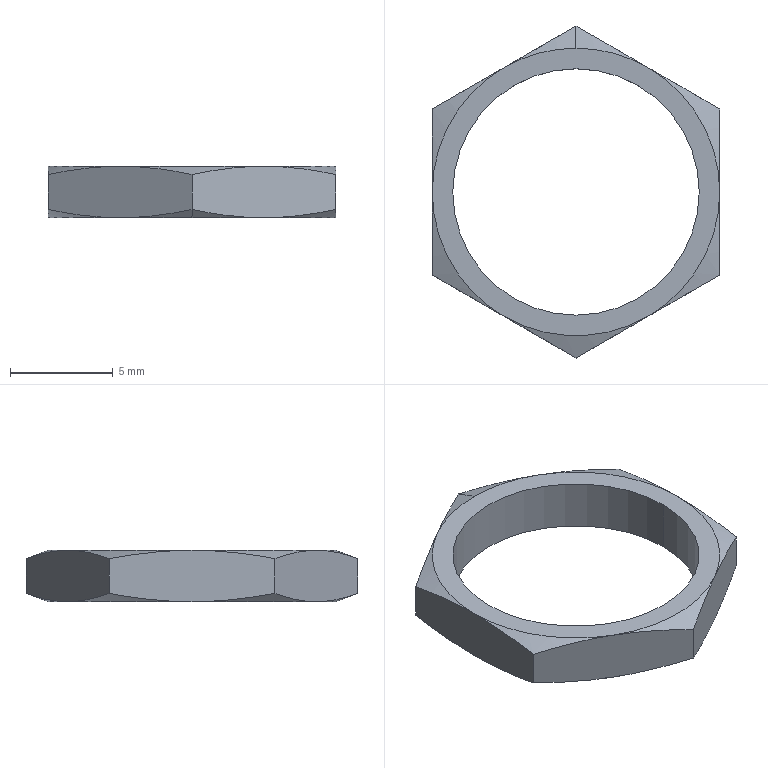Part | SolidWorks | features Extrusion 1, RevCut 1 | 1 solid | 24 faces | box 14 x 16.166 x 2.5 mm | volume 137.79 mm3 | cone 14 | plane 8 | cylinder 2 | commonest cylinder face diameters 12 x2
STEP:
#1=CARTESIAN_POINT('',(-3.5,6.062,2.5));
#2=VERTEX_POINT('',#1);
#3=CARTESIAN_POINT('',(0.,7.,2.5));
#4=VERTEX_POINT('',#3);
#5=CARTESIAN_POINT('',(0.,0.,2.5));
#6=DIRECTION('',(0.,0.,-1.));
#7=DIRECTION('',(0.,1.,0.));
#8=AXIS2_PLACEMENT_3D('',#5,#6,#7);
#9=CIRCLE('',#8,7.);
#10=EDGE_CURVE('',#2,#4,#9,.T.);
#11=ORIENTED_EDGE('',*,*,#10,.T.);
#12=CARTESIAN_POINT('',(0.,8.083,2.1));
#13=VERTEX_POINT('',#12);
#14=CARTESIAN_POINT('',(0.,7.,2.5));
#15=DIRECTION('',(0.,0.9381,-0.3465));
#16=VECTOR('',#15,1000.);
#17=LINE('',#14,#16);
#18=EDGE_CURVE('',#4,#13,#17,.T.);
#19=ORIENTED_EDGE('',*,*,#18,.T.);
#20=CARTESIAN_POINT('',(-3.5,6.062,2.5));
#21=CARTESIAN_POINT('',(-2.917,6.399,2.5));
#22=CARTESIAN_POINT('',(-2.333,6.736,2.463));
#23=CARTESIAN_POINT('',(-1.167,7.409,2.325));
#24=CARTESIAN_POINT('',(-0.5833,7.746,2.224));
#25=CARTESIAN_POINT('',(0.,8.083,2.1));
#26=B_SPLINE_CURVE_WITH_KNOTS('',3,(#20,#21,#22,#23,#24,#25),.UNSPECIFIED.,.F.,.F.,(4,2,4),(0.004042,0.006062,0.008083),.UNSPECIFIED.);
#27=EDGE_CURVE('',#2,#13,#26,.T.);
#28=ORIENTED_EDGE('',*,*,#27,.F.);
#29=EDGE_LOOP('',(#11,#19,#28));
#30=FACE_OUTER_BOUND('',#29,.T.);
#31=CARTESIAN_POINT('',(0.,0.,2.5));
#32=DIRECTION('',(0.,0.,-1.));
#33=DIRECTION('',(0.,1.,0.));
#34=AXIS2_PLACEMENT_3D('',#31,#32,#33);
#35=CONICAL_SURFACE('',#34,7.,1.217);
#36=ADVANCED_FACE('',(#30),#35,.T.);
#37=CARTESIAN_POINT('',(0.,-7.,0.));
#38=VERTEX_POINT('',#37);
#39=CARTESIAN_POINT('',(-3.5,-6.062,0.));
#40=VERTEX_POINT('',#39);
#41=CARTESIAN_POINT('',(0.,0.,0.));
#42=DIRECTION('',(0.,0.,-1.));
#43=DIRECTION('',(0.,1.,0.));
#44=AXIS2_PLACEMENT_3D('',#41,#42,#43);
#45=CIRCLE('',#44,7.);
#46=EDGE_CURVE('',#38,#40,#45,.T.);
#47=ORIENTED_EDGE('',*,*,#46,.F.);
#48=CARTESIAN_POINT('',(0.,-8.083,0.4));
#49=VERTEX_POINT('',#48);
#50=CARTESIAN_POINT('',(0.,-8.083,0.4));
#51=DIRECTION('',(0.,-0.9381,0.3465));
#52=VECTOR('',#51,1000.);
#53=LINE('',#50,#52);
#54=EDGE_CURVE('',#38,#49,#53,.T.);
#55=ORIENTED_EDGE('',*,*,#54,.T.);
#56=CARTESIAN_POINT('',(-3.5,-6.062,0.));
#57=CARTESIAN_POINT('',(-2.917,-6.399,0.));
#58=CARTESIAN_POINT('',(-2.333,-6.736,0.03657));
#59=CARTESIAN_POINT('',(-1.167,-7.409,0.1746));
#60=CARTESIAN_POINT('',(-0.5833,-7.746,0.2756));
#61=CARTESIAN_POINT('',(0.,-8.083,0.4));
#62=B_SPLINE_CURVE_WITH_KNOTS('',3,(#56,#57,#58,#59,#60,#61),.UNSPECIFIED.,.F.,.F.,(4,2,4),(0.004042,0.006062,0.008083),.UNSPECIFIED.);
#63=EDGE_CURVE('',#40,#49,#62,.T.);
#64=ORIENTED_EDGE('',*,*,#63,.F.);
#65=EDGE_LOOP('',(#47,#55,#64));
#66=FACE_OUTER_BOUND('',#65,.T.);
#67=CARTESIAN_POINT('',(0.,0.,0.4));
#68=DIRECTION('',(0.,0.,1.));
#69=DIRECTION('',(0.,-1.,0.));
#70=AXIS2_PLACEMENT_3D('',#67,#68,#69);
#71=CONICAL_SURFACE('',#70,8.083,1.217);
#72=ADVANCED_FACE('',(#66),#71,.T.);
#73=CARTESIAN_POINT('',(-6.,0.,2.5));
#74=VERTEX_POINT('',#73);
#75=CARTESIAN_POINT('',(6.,0.,2.5));
#76=VERTEX_POINT('',#75);
#77=CARTESIAN_POINT('',(0.,0.,2.5));
#78=DIRECTION('',(0.,0.,1.));
#79=DIRECTION('',(1.,0.,0.));
#80=AXIS2_PLACEMENT_3D('',#77,#78,#79);
#81=CIRCLE('',#80,6.);
#82=EDGE_CURVE('',#74,#76,#81,.T.);
#83=ORIENTED_EDGE('',*,*,#82,.T.);
#84=CARTESIAN_POINT('',(6.,0.,0.));
#85=VERTEX_POINT('',#84);
#86=CARTESIAN_POINT('',(6.,0.,2.5));
#87=DIRECTION('',(0.,0.,-1.));
#88=VECTOR('',#87,1000.);
#89=LINE('',#86,#88);
#90=EDGE_CURVE('',#76,#85,#89,.T.);
#91=ORIENTED_EDGE('',*,*,#90,.T.);
#92=CARTESIAN_POINT('',(-6.,0.,0.));
#93=VERTEX_POINT('',#92);
#94=CARTESIAN_POINT('',(0.,0.,0.));
#95=DIRECTION('',(0.,0.,1.));
#96=DIRECTION('',(1.,0.,0.));
#97=AXIS2_PLACEMENT_3D('',#94,#95,#96);
#98=CIRCLE('',#97,6.);
#99=EDGE_CURVE('',#93,#85,#98,.T.);
#100=ORIENTED_EDGE('',*,*,#99,.F.);
#101=CARTESIAN_POINT('',(-6.,0.,2.5));
#102=DIRECTION('',(0.,0.,-1.));
#103=VECTOR('',#102,1000.);
#104=LINE('',#101,#103);
#105=EDGE_CURVE('',#74,#93,#104,.T.);
#106=ORIENTED_EDGE('',*,*,#105,.F.);
#107=EDGE_LOOP('',(#83,#91,#100,#106));
#108=FACE_OUTER_BOUND('',#107,.T.);
#109=CARTESIAN_POINT('',(0.,0.,2.5));
#110=DIRECTION('',(0.,0.,-1.));
#111=DIRECTION('',(-1.,0.,0.));
#112=AXIS2_PLACEMENT_3D('',#109,#110,#111);
#113=CYLINDRICAL_SURFACE('',#112,6.);
#114=ADVANCED_FACE('',(#108),#113,.F.);
#115=ORIENTED_EDGE('',*,*,#82,.F.);
#116=CARTESIAN_POINT('',(0.,0.,2.5));
#117=DIRECTION('',(0.,0.,1.));
#118=DIRECTION('',(1.,0.,0.));
#119=AXIS2_PLACEMENT_3D('',#116,#117,#118);
#120=CIRCLE('',#119,6.);
#121=EDGE_CURVE('',#76,#74,#120,.T.);
#122=ORIENTED_EDGE('',*,*,#121,.F.);
#123=EDGE_LOOP('',(#115,#122));
#124=FACE_BOUND('',#123,.T.);
#125=CARTESIAN_POINT('',(7.,0.,2.5));
#126=VERTEX_POINT('',#125);
#127=CARTESIAN_POINT('',(3.5,-6.062,2.5));
#128=VERTEX_POINT('',#127);
#129=CARTESIAN_POINT('',(0.,0.,2.5));
#130=DIRECTION('',(0.,0.,-1.));
#131=DIRECTION('',(0.,1.,0.));
#132=AXIS2_PLACEMENT_3D('',#129,#130,#131);
#133=CIRCLE('',#132,7.);
#134=EDGE_CURVE('',#126,#128,#133,.T.);
#135=ORIENTED_EDGE('',*,*,#134,.F.);
#136=CARTESIAN_POINT('',(3.5,6.062,2.5));
#137=VERTEX_POINT('',#136);
#138=CARTESIAN_POINT('',(0.,0.,2.5));
#139=DIRECTION('',(0.,0.,-1.));
#140=DIRECTION('',(0.,1.,0.));
#141=AXIS2_PLACEMENT_3D('',#138,#139,#140);
#142=CIRCLE('',#141,7.);
#143=EDGE_CURVE('',#137,#126,#142,.T.);
#144=ORIENTED_EDGE('',*,*,#143,.F.);
#145=CARTESIAN_POINT('',(0.,0.,2.5));
#146=DIRECTION('',(0.,0.,-1.));
#147=DIRECTION('',(0.,1.,0.));
#148=AXIS2_PLACEMENT_3D('',#145,#146,#147);
#149=CIRCLE('',#148,7.);
#150=EDGE_CURVE('',#4,#137,#149,.T.);
#151=ORIENTED_EDGE('',*,*,#150,.F.);
#152=ORIENTED_EDGE('',*,*,#10,.F.);
#153=CARTESIAN_POINT('',(-7.,0.,2.5));
#154=VERTEX_POINT('',#153);
#155=CARTESIAN_POINT('',(0.,0.,2.5));
#156=DIRECTION('',(0.,0.,-1.));
#157=DIRECTION('',(0.,1.,0.));
#158=AXIS2_PLACEMENT_3D('',#155,#156,#157);
#159=CIRCLE('',#158,7.);
#160=EDGE_CURVE('',#154,#2,#159,.T.);
#161=ORIENTED_EDGE('',*,*,#160,.F.);
#162=CARTESIAN_POINT('',(-3.5,-6.062,2.5));
#163=VERTEX_POINT('',#162);
#164=CARTESIAN_POINT('',(0.,0.,2.5));
#165=DIRECTION('',(0.,0.,-1.));
#166=DIRECTION('',(0.,1.,0.));
#167=AXIS2_PLACEMENT_3D('',#164,#165,#166);
#168=CIRCLE('',#167,7.);
#169=EDGE_CURVE('',#163,#154,#168,.T.);
#170=ORIENTED_EDGE('',*,*,#169,.F.);
#171=CARTESIAN_POINT('',(0.,0.,2.5));
#172=DIRECTION('',(0.,0.,-1.));
#173=DIRECTION('',(0.,1.,0.));
#174=AXIS2_PLACEMENT_3D('',#171,#172,#173);
#175=CIRCLE('',#174,7.);
#176=EDGE_CURVE('',#128,#163,#175,.T.);
#177=ORIENTED_EDGE('',*,*,#176,.F.);
#178=EDGE_LOOP('',(#135,#144,#151,#152,#161,#170,#177));
#179=FACE_OUTER_BOUND('',#178,.T.);
#180=CARTESIAN_POINT('',(0.,0.,2.5));
#181=DIRECTION('',(0.,0.,1.));
#182=DIRECTION('',(1.,0.,0.));
#183=AXIS2_PLACEMENT_3D('',#180,#181,#182);
#184=PLANE('',#183);
#185=ADVANCED_FACE('',(#124,#179),#184,.T.);
#186=CARTESIAN_POINT('',(3.5,6.062,0.));
#187=VERTEX_POINT('',#186);
#188=CARTESIAN_POINT('',(7.,0.,0.));
#189=VERTEX_POINT('',#188);
#190=CARTESIAN_POINT('',(0.,0.,0.));
#191=DIRECTION('',(0.,0.,-1.));
#192=DIRECTION('',(0.,1.,0.));
#193=AXIS2_PLACEMENT_3D('',#190,#191,#192);
#194=CIRCLE('',#193,7.);
#195=EDGE_CURVE('',#187,#189,#194,.T.);
#196=ORIENTED_EDGE('',*,*,#195,.T.);
#197=CARTESIAN_POINT('',(3.5,-6.062,0.));
#198=VERTEX_POINT('',#197);
#199=CARTESIAN_POINT('',(0.,0.,0.));
#200=DIRECTION('',(0.,0.,-1.));
#201=DIRECTION('',(0.,1.,0.));
#202=AXIS2_PLACEMENT_3D('',#199,#200,#201);
#203=CIRCLE('',#202,7.);
#204=EDGE_CURVE('',#189,#198,#203,.T.);
#205=ORIENTED_EDGE('',*,*,#204,.T.);
#206=CARTESIAN_POINT('',(0.,0.,0.));
#207=DIRECTION('',(0.,0.,-1.));
#208=DIRECTION('',(0.,1.,0.));
#209=AXIS2_PLACEMENT_3D('',#206,#207,#208);
#210=CIRCLE('',#209,7.);
#211=EDGE_CURVE('',#198,#38,#210,.T.);
#212=ORIENTED_EDGE('',*,*,#211,.T.);
#213=ORIENTED_EDGE('',*,*,#46,.T.);
#214=CARTESIAN_POINT('',(-7.,0.,0.));
#215=VERTEX_POINT('',#214);
#216=CARTESIAN_POINT('',(0.,0.,0.));
#217=DIRECTION('',(0.,0.,-1.));
#218=DIRECTION('',(0.,1.,0.));
#219=AXIS2_PLACEMENT_3D('',#216,#217,#218);
#220=CIRCLE('',#219,7.);
#221=EDGE_CURVE('',#40,#215,#220,.T.);
#222=ORIENTED_EDGE('',*,*,#221,.T.);
#223=CARTESIAN_POINT('',(-3.5,6.062,0.));
#224=VERTEX_POINT('',#223);
#225=CARTESIAN_POINT('',(0.,0.,0.));
#226=DIRECTION('',(0.,0.,-1.));
#227=DIRECTION('',(0.,1.,0.));
#228=AXIS2_PLACEMENT_3D('',#225,#226,#227);
#229=CIRCLE('',#228,7.);
#230=EDGE_CURVE('',#215,#224,#229,.T.);
#231=ORIENTED_EDGE('',*,*,#230,.T.);
#232=CARTESIAN_POINT('',(0.,0.,0.));
#233=DIRECTION('',(0.,0.,-1.));
#234=DIRECTION('',(0.,1.,0.));
#235=AXIS2_PLACEMENT_3D('',#232,#233,#234);
#236=CIRCLE('',#235,7.);
#237=EDGE_CURVE('',#224,#187,#236,.T.);
#238=ORIENTED_EDGE('',*,*,#237,.T.);
#239=EDGE_LOOP('',(#196,#205,#212,#213,#222,#231,#238));
#240=FACE_OUTER_BOUND('',#239,.T.);
#241=ORIENTED_EDGE('',*,*,#99,.T.);
#242=CARTESIAN_POINT('',(0.,0.,0.));
#243=DIRECTION('',(0.,0.,1.));
#244=DIRECTION('',(1.,0.,0.));
#245=AXIS2_PLACEMENT_3D('',#242,#243,#244);
#246=CIRCLE('',#245,6.);
#247=EDGE_CURVE('',#85,#93,#246,.T.);
#248=ORIENTED_EDGE('',*,*,#247,.T.);
#249=EDGE_LOOP('',(#241,#248));
#250=FACE_BOUND('',#249,.T.);
#251=CARTESIAN_POINT('',(0.,0.,0.));
#252=DIRECTION('',(0.,0.,1.));
#253=DIRECTION('',(1.,0.,0.));
#254=AXIS2_PLACEMENT_3D('',#251,#252,#253);
#255=PLANE('',#254);
#256=ADVANCED_FACE('',(#240,#250),#255,.F.);
#257=ORIENTED_EDGE('',*,*,#90,.F.);
#258=ORIENTED_EDGE('',*,*,#121,.T.);
#259=ORIENTED_EDGE('',*,*,#105,.T.);
#260=ORIENTED_EDGE('',*,*,#247,.F.);
#261=EDGE_LOOP('',(#257,#258,#259,#260));
#262=FACE_OUTER_BOUND('',#261,.T.);
#263=CARTESIAN_POINT('',(0.,0.,2.5));
#264=DIRECTION('',(0.,0.,-1.));
#265=DIRECTION('',(-1.,0.,0.));
#266=AXIS2_PLACEMENT_3D('',#263,#264,#265);
#267=CYLINDRICAL_SURFACE('',#266,6.);
#268=ADVANCED_FACE('',(#262),#267,.F.);
#269=CARTESIAN_POINT('',(7.,-4.041,2.1));
#270=VERTEX_POINT('',#269);
#271=CARTESIAN_POINT('',(7.,0.,2.5));
#272=CARTESIAN_POINT('',(7.,-0.6732,2.5));
#273=CARTESIAN_POINT('',(7.,-1.347,2.463));
#274=CARTESIAN_POINT('',(7.,-2.696,2.325));
#275=CARTESIAN_POINT('',(7.,-3.373,2.224));
#276=CARTESIAN_POINT('',(7.,-4.041,2.1));
#277=B_SPLINE_CURVE_WITH_KNOTS('',3,(#271,#272,#273,#274,#275,#276),.UNSPECIFIED.,.F.,.F.,(4,2,4),(0.01855,0.02058,0.02262),.UNSPECIFIED.);
#278=EDGE_CURVE('',#126,#270,#277,.T.);
#279=ORIENTED_EDGE('',*,*,#278,.F.);
#280=ORIENTED_EDGE('',*,*,#134,.T.);
#281=CARTESIAN_POINT('',(7.,-4.041,2.1));
#282=CARTESIAN_POINT('',(6.417,-4.378,2.224));
#283=CARTESIAN_POINT('',(5.833,-4.715,2.325));
#284=CARTESIAN_POINT('',(4.667,-5.389,2.463));
#285=CARTESIAN_POINT('',(4.083,-5.725,2.5));
#286=CARTESIAN_POINT('',(3.5,-6.062,2.5));
#287=B_SPLINE_CURVE_WITH_KNOTS('',3,(#281,#282,#283,#284,#285,#286),.UNSPECIFIED.,.F.,.F.,(4,2,4),(0.000000231,0.002021,0.004042),.UNSPECIFIED.);
#288=EDGE_CURVE('',#270,#128,#287,.T.);
#289=ORIENTED_EDGE('',*,*,#288,.F.);
#290=EDGE_LOOP('',(#279,#280,#289));
#291=FACE_OUTER_BOUND('',#290,.T.);
#292=CARTESIAN_POINT('',(0.,0.,2.5));
#293=DIRECTION('',(0.,0.,-1.));
#294=DIRECTION('',(0.,1.,0.));
#295=AXIS2_PLACEMENT_3D('',#292,#293,#294);
#296=CONICAL_SURFACE('',#295,7.,1.217);
#297=ADVANCED_FACE('',(#291),#296,.T.);
#298=ORIENTED_EDGE('',*,*,#143,.T.);
#299=CARTESIAN_POINT('',(7.,4.041,2.1));
#300=VERTEX_POINT('',#299);
#301=CARTESIAN_POINT('',(7.,4.041,2.1));
#302=CARTESIAN_POINT('',(7.,3.37,2.224));
#303=CARTESIAN_POINT('',(7.,2.696,2.325));
#304=CARTESIAN_POINT('',(7.,1.349,2.463));
#305=CARTESIAN_POINT('',(7.,0.6749,2.5));
#306=CARTESIAN_POINT('',(7.,0.,2.5));
#307=B_SPLINE_CURVE_WITH_KNOTS('',3,(#301,#302,#303,#304,#305,#306),.UNSPECIFIED.,.F.,.F.,(4,2,4),(0.01448,0.01652,0.01855),.UNSPECIFIED.);
#308=EDGE_CURVE('',#300,#126,#307,.T.);
#309=ORIENTED_EDGE('',*,*,#308,.F.);
#310=CARTESIAN_POINT('',(3.5,6.062,2.5));
#311=CARTESIAN_POINT('',(4.083,5.725,2.5));
#312=CARTESIAN_POINT('',(4.667,5.389,2.463));
#313=CARTESIAN_POINT('',(5.833,4.715,2.325));
#314=CARTESIAN_POINT('',(6.417,4.378,2.224));
#315=CARTESIAN_POINT('',(7.,4.041,2.1));
#316=B_SPLINE_CURVE_WITH_KNOTS('',3,(#310,#311,#312,#313,#314,#315),.UNSPECIFIED.,.F.,.F.,(4,2,4),(0.004042,0.006062,0.008083),.UNSPECIFIED.);
#317=EDGE_CURVE('',#137,#300,#316,.T.);
#318=ORIENTED_EDGE('',*,*,#317,.F.);
#319=EDGE_LOOP('',(#298,#309,#318));
#320=FACE_OUTER_BOUND('',#319,.T.);
#321=CARTESIAN_POINT('',(0.,0.,2.5));
#322=DIRECTION('',(0.,0.,-1.));
#323=DIRECTION('',(0.,1.,0.));
#324=AXIS2_PLACEMENT_3D('',#321,#322,#323);
#325=CONICAL_SURFACE('',#324,7.,1.217);
#326=ADVANCED_FACE('',(#320),#325,.T.);
#327=CARTESIAN_POINT('',(7.,4.041,0.4));
#328=VERTEX_POINT('',#327);
#329=CARTESIAN_POINT('',(7.,0.,0.));
#330=CARTESIAN_POINT('',(7.,0.6749,0.));
#331=CARTESIAN_POINT('',(7.,1.349,0.03671));
#332=CARTESIAN_POINT('',(7.,2.696,0.1748));
#333=CARTESIAN_POINT('',(7.,3.37,0.276));
#334=CARTESIAN_POINT('',(7.,4.041,0.4));
#335=B_SPLINE_CURVE_WITH_KNOTS('',3,(#329,#330,#331,#332,#333,#334),.UNSPECIFIED.,.F.,.F.,(4,2,4),(0.01096,0.013,0.01504),.UNSPECIFIED.);
#336=EDGE_CURVE('',#189,#328,#335,.T.);
#337=ORIENTED_EDGE('',*,*,#336,.F.);
#338=ORIENTED_EDGE('',*,*,#195,.F.);
#339=CARTESIAN_POINT('',(7.,4.041,0.4));
#340=CARTESIAN_POINT('',(6.417,4.378,0.2756));
#341=CARTESIAN_POINT('',(5.833,4.715,0.1746));
#342=CARTESIAN_POINT('',(4.667,5.389,0.03657));
#343=CARTESIAN_POINT('',(4.083,5.725,0.));
#344=CARTESIAN_POINT('',(3.5,6.062,0.));
#345=B_SPLINE_CURVE_WITH_KNOTS('',3,(#339,#340,#341,#342,#343,#344),.UNSPECIFIED.,.F.,.F.,(4,2,4),(0.000000231,0.002021,0.004042),.UNSPECIFIED.);
#346=EDGE_CURVE('',#328,#187,#345,.T.);
#347=ORIENTED_EDGE('',*,*,#346,.F.);
#348=EDGE_LOOP('',(#337,#338,#347));
#349=FACE_OUTER_BOUND('',#348,.T.);
#350=CARTESIAN_POINT('',(0.,0.,0.4));
#351=DIRECTION('',(0.,0.,1.));
#352=DIRECTION('',(0.,-1.,0.));
#353=AXIS2_PLACEMENT_3D('',#350,#351,#352);
#354=CONICAL_SURFACE('',#353,8.083,1.217);
#355=ADVANCED_FACE('',(#349),#354,.T.);
#356=ORIENTED_EDGE('',*,*,#204,.F.);
#357=CARTESIAN_POINT('',(7.,-4.041,0.4));
#358=VERTEX_POINT('',#357);
#359=CARTESIAN_POINT('',(7.,-4.041,0.4));
#360=CARTESIAN_POINT('',(7.,-3.373,0.2765));
#361=CARTESIAN_POINT('',(7.,-2.696,0.1748));
#362=CARTESIAN_POINT('',(7.,-1.347,0.03654));
#363=CARTESIAN_POINT('',(7.,-0.6732,0.));
#364=CARTESIAN_POINT('',(7.,0.,0.));
#365=B_SPLINE_CURVE_WITH_KNOTS('',3,(#359,#360,#361,#362,#363,#364),.UNSPECIFIED.,.F.,.F.,(4,2,4),(0.006882,0.008919,0.01096),.UNSPECIFIED.);
#366=EDGE_CURVE('',#358,#189,#365,.T.);
#367=ORIENTED_EDGE('',*,*,#366,.F.);
#368=CARTESIAN_POINT('',(3.5,-6.062,0.));
#369=CARTESIAN_POINT('',(4.083,-5.725,0.));
#370=CARTESIAN_POINT('',(4.667,-5.389,0.03657));
#371=CARTESIAN_POINT('',(5.833,-4.715,0.1746));
#372=CARTESIAN_POINT('',(6.417,-4.378,0.2756));
#373=CARTESIAN_POINT('',(7.,-4.041,0.4));
#374=B_SPLINE_CURVE_WITH_KNOTS('',3,(#368,#369,#370,#371,#372,#373),.UNSPECIFIED.,.F.,.F.,(4,2,4),(0.004042,0.006062,0.008083),.UNSPECIFIED.);
#375=EDGE_CURVE('',#198,#358,#374,.T.);
#376=ORIENTED_EDGE('',*,*,#375,.F.);
#377=EDGE_LOOP('',(#356,#367,#376));
#378=FACE_OUTER_BOUND('',#377,.T.);
#379=CARTESIAN_POINT('',(0.,0.,0.4));
#380=DIRECTION('',(0.,0.,1.));
#381=DIRECTION('',(0.,-1.,0.));
#382=AXIS2_PLACEMENT_3D('',#379,#380,#381);
#383=CONICAL_SURFACE('',#382,8.083,1.217);
#384=ADVANCED_FACE('',(#378),#383,.T.);
#385=CARTESIAN_POINT('',(0.,-8.083,2.1));
#386=VERTEX_POINT('',#385);
#387=CARTESIAN_POINT('',(3.5,-6.062,2.5));
#388=CARTESIAN_POINT('',(2.917,-6.399,2.5));
#389=CARTESIAN_POINT('',(2.333,-6.736,2.463));
#390=CARTESIAN_POINT('',(1.167,-7.409,2.325));
#391=CARTESIAN_POINT('',(0.5833,-7.746,2.224));
#392=CARTESIAN_POINT('',(0.,-8.083,2.1));
#393=B_SPLINE_CURVE_WITH_KNOTS('',3,(#387,#388,#389,#390,#391,#392),.UNSPECIFIED.,.F.,.F.,(4,2,4),(0.004042,0.006062,0.008083),.UNSPECIFIED.);
#394=EDGE_CURVE('',#128,#386,#393,.T.);
#395=ORIENTED_EDGE('',*,*,#394,.F.);
#396=ORIENTED_EDGE('',*,*,#176,.T.);
#397=CARTESIAN_POINT('',(0.,-8.083,2.1));
#398=CARTESIAN_POINT('',(-0.5833,-7.746,2.224));
#399=CARTESIAN_POINT('',(-1.167,-7.409,2.325));
#400=CARTESIAN_POINT('',(-2.333,-6.736,2.463));
#401=CARTESIAN_POINT('',(-2.917,-6.399,2.5));
#402=CARTESIAN_POINT('',(-3.5,-6.062,2.5));
#403=B_SPLINE_CURVE_WITH_KNOTS('',3,(#397,#398,#399,#400,#401,#402),.UNSPECIFIED.,.F.,.F.,(4,2,4),(0.000000231,0.002021,0.004042),.UNSPECIFIED.);
#404=EDGE_CURVE('',#386,#163,#403,.T.);
#405=ORIENTED_EDGE('',*,*,#404,.F.);
#406=EDGE_LOOP('',(#395,#396,#405));
#407=FACE_OUTER_BOUND('',#406,.T.);
#408=CARTESIAN_POINT('',(0.,0.,2.5));
#409=DIRECTION('',(0.,0.,-1.));
#410=DIRECTION('',(0.,1.,0.));
#411=AXIS2_PLACEMENT_3D('',#408,#409,#410);
#412=CONICAL_SURFACE('',#411,7.,1.217);
#413=ADVANCED_FACE('',(#407),#412,.T.);
#414=ORIENTED_EDGE('',*,*,#54,.F.);
#415=ORIENTED_EDGE('',*,*,#211,.F.);
#416=CARTESIAN_POINT('',(0.,-8.083,0.4));
#417=CARTESIAN_POINT('',(0.5833,-7.746,0.2756));
#418=CARTESIAN_POINT('',(1.167,-7.409,0.1746));
#419=CARTESIAN_POINT('',(2.333,-6.736,0.03657));
#420=CARTESIAN_POINT('',(2.917,-6.399,0.));
#421=CARTESIAN_POINT('',(3.5,-6.062,0.));
#422=B_SPLINE_CURVE_WITH_KNOTS('',3,(#416,#417,#418,#419,#420,#421),.UNSPECIFIED.,.F.,.F.,(4,2,4),(0.000000231,0.002021,0.004042),.UNSPECIFIED.);
#423=EDGE_CURVE('',#49,#198,#422,.T.);
#424=ORIENTED_EDGE('',*,*,#423,.F.);
#425=EDGE_LOOP('',(#414,#415,#424));
#426=FACE_OUTER_BOUND('',#425,.T.);
#427=CARTESIAN_POINT('',(0.,0.,0.4));
#428=DIRECTION('',(0.,0.,1.));
#429=DIRECTION('',(0.,-1.,0.));
#430=AXIS2_PLACEMENT_3D('',#427,#428,#429);
#431=CONICAL_SURFACE('',#430,8.083,1.217);
#432=ADVANCED_FACE('',(#426),#431,.T.);
#433=CARTESIAN_POINT('',(-7.,-4.041,2.1));
#434=VERTEX_POINT('',#433);
#435=CARTESIAN_POINT('',(-3.5,-6.062,2.5));
#436=CARTESIAN_POINT('',(-4.083,-5.725,2.5));
#437=CARTESIAN_POINT('',(-4.667,-5.389,2.463));
#438=CARTESIAN_POINT('',(-5.833,-4.715,2.325));
#439=CARTESIAN_POINT('',(-6.417,-4.378,2.224));
#440=CARTESIAN_POINT('',(-7.,-4.041,2.1));
#441=B_SPLINE_CURVE_WITH_KNOTS('',3,(#435,#436,#437,#438,#439,#440),.UNSPECIFIED.,.F.,.F.,(4,2,4),(0.004042,0.006062,0.008083),.UNSPECIFIED.);
#442=EDGE_CURVE('',#163,#434,#441,.T.);
#443=ORIENTED_EDGE('',*,*,#442,.F.);
#444=ORIENTED_EDGE('',*,*,#169,.T.);
#445=CARTESIAN_POINT('',(-7.,-4.041,2.1));
#446=CARTESIAN_POINT('',(-7.,-3.373,2.224));
#447=CARTESIAN_POINT('',(-7.,-2.696,2.325));
#448=CARTESIAN_POINT('',(-7.,-1.347,2.463));
#449=CARTESIAN_POINT('',(-7.,-0.6732,2.5));
#450=CARTESIAN_POINT('',(-7.,0.,2.5));
#451=B_SPLINE_CURVE_WITH_KNOTS('',3,(#445,#446,#447,#448,#449,#450),.UNSPECIFIED.,.F.,.F.,(4,2,4),(0.006882,0.008919,0.01096),.UNSPECIFIED.);
#452=EDGE_CURVE('',#434,#154,#451,.T.);
#453=ORIENTED_EDGE('',*,*,#452,.F.);
#454=EDGE_LOOP('',(#443,#444,#453));
#455=FACE_OUTER_BOUND('',#454,.T.);
#456=CARTESIAN_POINT('',(0.,0.,2.5));
#457=DIRECTION('',(0.,0.,-1.));
#458=DIRECTION('',(0.,1.,0.));
#459=AXIS2_PLACEMENT_3D('',#456,#457,#458);
#460=CONICAL_SURFACE('',#459,7.,1.217);
#461=ADVANCED_FACE('',(#455),#460,.T.);
#462=ORIENTED_EDGE('',*,*,#221,.F.);
#463=CARTESIAN_POINT('',(-7.,-4.041,0.4));
#464=VERTEX_POINT('',#463);
#465=CARTESIAN_POINT('',(-7.,-4.041,0.4));
#466=CARTESIAN_POINT('',(-6.417,-4.378,0.2756));
#467=CARTESIAN_POINT('',(-5.833,-4.715,0.1746));
#468=CARTESIAN_POINT('',(-4.667,-5.389,0.03657));
#469=CARTESIAN_POINT('',(-4.083,-5.725,0.));
#470=CARTESIAN_POINT('',(-3.5,-6.062,0.));
#471=B_SPLINE_CURVE_WITH_KNOTS('',3,(#465,#466,#467,#468,#469,#470),.UNSPECIFIED.,.F.,.F.,(4,2,4),(0.000000231,0.002021,0.004042),.UNSPECIFIED.);
#472=EDGE_CURVE('',#464,#40,#471,.T.);
#473=ORIENTED_EDGE('',*,*,#472,.F.);
#474=CARTESIAN_POINT('',(-7.,0.,0.));
#475=CARTESIAN_POINT('',(-7.,-0.6732,0.));
#476=CARTESIAN_POINT('',(-7.,-1.347,0.03654));
#477=CARTESIAN_POINT('',(-7.,-2.696,0.1748));
#478=CARTESIAN_POINT('',(-7.,-3.373,0.2765));
#479=CARTESIAN_POINT('',(-7.,-4.041,0.4));
#480=B_SPLINE_CURVE_WITH_KNOTS('',3,(#474,#475,#476,#477,#478,#479),.UNSPECIFIED.,.F.,.F.,(4,2,4),(0.01855,0.02058,0.02262),.UNSPECIFIED.);
#481=EDGE_CURVE('',#215,#464,#480,.T.);
#482=ORIENTED_EDGE('',*,*,#481,.F.);
#483=EDGE_LOOP('',(#462,#473,#482));
#484=FACE_OUTER_BOUND('',#483,.T.);
#485=CARTESIAN_POINT('',(0.,0.,0.4));
#486=DIRECTION('',(0.,0.,1.));
#487=DIRECTION('',(0.,-1.,0.));
#488=AXIS2_PLACEMENT_3D('',#485,#486,#487);
#489=CONICAL_SURFACE('',#488,8.083,1.217);
#490=ADVANCED_FACE('',(#484),#489,.T.);
#491=ORIENTED_EDGE('',*,*,#160,.T.);
#492=CARTESIAN_POINT('',(-7.,4.041,2.1));
#493=VERTEX_POINT('',#492);
#494=CARTESIAN_POINT('',(-7.,4.041,2.1));
#495=CARTESIAN_POINT('',(-6.417,4.378,2.224));
#496=CARTESIAN_POINT('',(-5.833,4.715,2.325));
#497=CARTESIAN_POINT('',(-4.667,5.389,2.463));
#498=CARTESIAN_POINT('',(-4.083,5.725,2.5));
#499=CARTESIAN_POINT('',(-3.5,6.062,2.5));
#500=B_SPLINE_CURVE_WITH_KNOTS('',3,(#494,#495,#496,#497,#498,#499),.UNSPECIFIED.,.F.,.F.,(4,2,4),(0.000000231,0.002021,0.004042),.UNSPECIFIED.);
#501=EDGE_CURVE('',#493,#2,#500,.T.);
#502=ORIENTED_EDGE('',*,*,#501,.F.);
#503=CARTESIAN_POINT('',(-7.,0.,2.5));
#504=CARTESIAN_POINT('',(-7.,0.6749,2.5));
#505=CARTESIAN_POINT('',(-7.,1.349,2.463));
#506=CARTESIAN_POINT('',(-7.,2.696,2.325));
#507=CARTESIAN_POINT('',(-7.,3.37,2.224));
#508=CARTESIAN_POINT('',(-7.,4.041,2.1));
#509=B_SPLINE_CURVE_WITH_KNOTS('',3,(#503,#504,#505,#506,#507,#508),.UNSPECIFIED.,.F.,.F.,(4,2,4),(0.01096,0.013,0.01504),.UNSPECIFIED.);
#510=EDGE_CURVE('',#154,#493,#509,.T.);
#511=ORIENTED_EDGE('',*,*,#510,.F.);
#512=EDGE_LOOP('',(#491,#502,#511));
#513=FACE_OUTER_BOUND('',#512,.T.);
#514=CARTESIAN_POINT('',(0.,0.,2.5));
#515=DIRECTION('',(0.,0.,-1.));
#516=DIRECTION('',(0.,1.,0.));
#517=AXIS2_PLACEMENT_3D('',#514,#515,#516);
#518=CONICAL_SURFACE('',#517,7.,1.217);
#519=ADVANCED_FACE('',(#513),#518,.T.);
#520=ORIENTED_EDGE('',*,*,#230,.F.);
#521=CARTESIAN_POINT('',(-7.,4.041,0.4));
#522=VERTEX_POINT('',#521);
#523=CARTESIAN_POINT('',(-7.,4.041,0.4));
#524=CARTESIAN_POINT('',(-7.,3.37,0.276));
#525=CARTESIAN_POINT('',(-7.,2.696,0.1748));
#526=CARTESIAN_POINT('',(-7.,1.349,0.03671));
#527=CARTESIAN_POINT('',(-7.,0.6749,0.));
#528=CARTESIAN_POINT('',(-7.,0.,0.));
#529=B_SPLINE_CURVE_WITH_KNOTS('',3,(#523,#524,#525,#526,#527,#528),.UNSPECIFIED.,.F.,.F.,(4,2,4),(0.01448,0.01652,0.01855),.UNSPECIFIED.);
#530=EDGE_CURVE('',#522,#215,#529,.T.);
#531=ORIENTED_EDGE('',*,*,#530,.F.);
#532=CARTESIAN_POINT('',(-3.5,6.062,0.));
#533=CARTESIAN_POINT('',(-4.083,5.725,0.));
#534=CARTESIAN_POINT('',(-4.667,5.389,0.03657));
#535=CARTESIAN_POINT('',(-5.833,4.715,0.1746));
#536=CARTESIAN_POINT('',(-6.417,4.378,0.2756));
#537=CARTESIAN_POINT('',(-7.,4.041,0.4));
#538=B_SPLINE_CURVE_WITH_KNOTS('',3,(#532,#533,#534,#535,#536,#537),.UNSPECIFIED.,.F.,.F.,(4,2,4),(0.004042,0.006062,0.008083),.UNSPECIFIED.);
#539=EDGE_CURVE('',#224,#522,#538,.T.);
#540=ORIENTED_EDGE('',*,*,#539,.F.);
#541=EDGE_LOOP('',(#520,#531,#540));
#542=FACE_OUTER_BOUND('',#541,.T.);
#543=CARTESIAN_POINT('',(0.,0.,0.4));
#544=DIRECTION('',(0.,0.,1.));
#545=DIRECTION('',(0.,-1.,0.));
#546=AXIS2_PLACEMENT_3D('',#543,#544,#545);
#547=CONICAL_SURFACE('',#546,8.083,1.217);
#548=ADVANCED_FACE('',(#542),#547,.T.);
#549=ORIENTED_EDGE('',*,*,#18,.F.);
#550=ORIENTED_EDGE('',*,*,#150,.T.);
#551=CARTESIAN_POINT('',(0.,8.083,2.1));
#552=CARTESIAN_POINT('',(0.5833,7.746,2.224));
#553=CARTESIAN_POINT('',(1.167,7.409,2.325));
#554=CARTESIAN_POINT('',(2.333,6.736,2.463));
#555=CARTESIAN_POINT('',(2.917,6.399,2.5));
#556=CARTESIAN_POINT('',(3.5,6.062,2.5));
#557=B_SPLINE_CURVE_WITH_KNOTS('',3,(#551,#552,#553,#554,#555,#556),.UNSPECIFIED.,.F.,.F.,(4,2,4),(0.000000231,0.002021,0.004042),.UNSPECIFIED.);
#558=EDGE_CURVE('',#13,#137,#557,.T.);
#559=ORIENTED_EDGE('',*,*,#558,.F.);
#560=EDGE_LOOP('',(#549,#550,#559));
#561=FACE_OUTER_BOUND('',#560,.T.);
#562=CARTESIAN_POINT('',(0.,0.,2.5));
#563=DIRECTION('',(0.,0.,-1.));
#564=DIRECTION('',(0.,1.,0.));
#565=AXIS2_PLACEMENT_3D('',#562,#563,#564);
#566=CONICAL_SURFACE('',#565,7.,1.217);
#567=ADVANCED_FACE('',(#561),#566,.T.);
#568=ORIENTED_EDGE('',*,*,#237,.F.);
#569=CARTESIAN_POINT('',(0.,8.083,0.4));
#570=VERTEX_POINT('',#569);
#571=CARTESIAN_POINT('',(0.,8.083,0.4));
#572=CARTESIAN_POINT('',(-0.5833,7.746,0.2756));
#573=CARTESIAN_POINT('',(-1.167,7.409,0.1746));
#574=CARTESIAN_POINT('',(-2.333,6.736,0.03657));
#575=CARTESIAN_POINT('',(-2.917,6.399,0.));
#576=CARTESIAN_POINT('',(-3.5,6.062,0.));
#577=B_SPLINE_CURVE_WITH_KNOTS('',3,(#571,#572,#573,#574,#575,#576),.UNSPECIFIED.,.F.,.F.,(4,2,4),(0.000000231,0.002021,0.004042),.UNSPECIFIED.);
#578=EDGE_CURVE('',#570,#224,#577,.T.);
#579=ORIENTED_EDGE('',*,*,#578,.F.);
#580=CARTESIAN_POINT('',(3.5,6.062,0.));
#581=CARTESIAN_POINT('',(2.917,6.399,0.));
#582=CARTESIAN_POINT('',(2.333,6.736,0.03657));
#583=CARTESIAN_POINT('',(1.167,7.409,0.1746));
#584=CARTESIAN_POINT('',(0.5833,7.746,0.2756));
#585=CARTESIAN_POINT('',(0.,8.083,0.4));
#586=B_SPLINE_CURVE_WITH_KNOTS('',3,(#580,#581,#582,#583,#584,#585),.UNSPECIFIED.,.F.,.F.,(4,2,4),(0.004042,0.006062,0.008083),.UNSPECIFIED.);
#587=EDGE_CURVE('',#187,#570,#586,.T.);
#588=ORIENTED_EDGE('',*,*,#587,.F.);
#589=EDGE_LOOP('',(#568,#579,#588));
#590=FACE_OUTER_BOUND('',#589,.T.);
#591=CARTESIAN_POINT('',(0.,0.,0.4));
#592=DIRECTION('',(0.,0.,1.));
#593=DIRECTION('',(0.,-1.,0.));
#594=AXIS2_PLACEMENT_3D('',#591,#592,#593);
#595=CONICAL_SURFACE('',#594,8.083,1.217);
#596=ADVANCED_FACE('',(#590),#595,.T.);
#597=CARTESIAN_POINT('',(7.,-4.041,2.5));
#598=DIRECTION('',(0.,0.,-1.));
#599=VECTOR('',#598,1000.);
#600=LINE('',#597,#599);
#601=EDGE_CURVE('',#270,#358,#600,.T.);
#602=ORIENTED_EDGE('',*,*,#601,.T.);
#603=ORIENTED_EDGE('',*,*,#366,.T.);
#604=ORIENTED_EDGE('',*,*,#336,.T.);
#605=CARTESIAN_POINT('',(7.,4.041,2.5));
#606=DIRECTION('',(0.,0.,-1.));
#607=VECTOR('',#606,1000.);
#608=LINE('',#605,#607);
#609=EDGE_CURVE('',#300,#328,#608,.T.);
#610=ORIENTED_EDGE('',*,*,#609,.F.);
#611=ORIENTED_EDGE('',*,*,#308,.T.);
#612=ORIENTED_EDGE('',*,*,#278,.T.);
#613=EDGE_LOOP('',(#602,#603,#604,#610,#611,#612));
#614=FACE_OUTER_BOUND('',#613,.T.);
#615=CARTESIAN_POINT('',(7.,-4.041,2.5));
#616=DIRECTION('',(-1.,0.,0.));
#617=DIRECTION('',(0.,-1.,0.));
#618=AXIS2_PLACEMENT_3D('',#615,#616,#617);
#619=PLANE('',#618);
#620=ADVANCED_FACE('',(#614),#619,.F.);
#621=CARTESIAN_POINT('',(0.,-8.083,2.5));
#622=DIRECTION('',(0.,0.,-1.));
#623=VECTOR('',#622,1000.);
#624=LINE('',#621,#623);
#625=EDGE_CURVE('',#386,#49,#624,.T.);
#626=ORIENTED_EDGE('',*,*,#625,.T.);
#627=ORIENTED_EDGE('',*,*,#423,.T.);
#628=ORIENTED_EDGE('',*,*,#375,.T.);
#629=ORIENTED_EDGE('',*,*,#601,.F.);
#630=ORIENTED_EDGE('',*,*,#288,.T.);
#631=ORIENTED_EDGE('',*,*,#394,.T.);
#632=EDGE_LOOP('',(#626,#627,#628,#629,#630,#631));
#633=FACE_OUTER_BOUND('',#632,.T.);
#634=CARTESIAN_POINT('',(0.,-8.083,2.5));
#635=DIRECTION('',(-0.5,0.866,0.));
#636=DIRECTION('',(-0.866,-0.5,0.));
#637=AXIS2_PLACEMENT_3D('',#634,#635,#636);
#638=PLANE('',#637);
#639=ADVANCED_FACE('',(#633),#638,.F.);
#640=CARTESIAN_POINT('',(-7.,-4.041,2.5));
#641=DIRECTION('',(0.,0.,-1.));
#642=VECTOR('',#641,1000.);
#643=LINE('',#640,#642);
#644=EDGE_CURVE('',#434,#464,#643,.T.);
#645=ORIENTED_EDGE('',*,*,#644,.T.);
#646=ORIENTED_EDGE('',*,*,#472,.T.);
#647=ORIENTED_EDGE('',*,*,#63,.T.);
#648=ORIENTED_EDGE('',*,*,#625,.F.);
#649=ORIENTED_EDGE('',*,*,#404,.T.);
#650=ORIENTED_EDGE('',*,*,#442,.T.);
#651=EDGE_LOOP('',(#645,#646,#647,#648,#649,#650));
#652=FACE_OUTER_BOUND('',#651,.T.);
#653=CARTESIAN_POINT('',(-7.,-4.041,2.5));
#654=DIRECTION('',(0.5,0.866,0.));
#655=DIRECTION('',(-0.866,0.5,0.));
#656=AXIS2_PLACEMENT_3D('',#653,#654,#655);
#657=PLANE('',#656);
#658=ADVANCED_FACE('',(#652),#657,.F.);
#659=CARTESIAN_POINT('',(-7.,4.041,2.5));
#660=DIRECTION('',(0.,0.,-1.));
#661=VECTOR('',#660,1000.);
#662=LINE('',#659,#661);
#663=EDGE_CURVE('',#493,#522,#662,.T.);
#664=ORIENTED_EDGE('',*,*,#663,.T.);
#665=ORIENTED_EDGE('',*,*,#530,.T.);
#666=ORIENTED_EDGE('',*,*,#481,.T.);
#667=ORIENTED_EDGE('',*,*,#644,.F.);
#668=ORIENTED_EDGE('',*,*,#452,.T.);
#669=ORIENTED_EDGE('',*,*,#510,.T.);
#670=EDGE_LOOP('',(#664,#665,#666,#667,#668,#669));
#671=FACE_OUTER_BOUND('',#670,.T.);
#672=CARTESIAN_POINT('',(-7.,4.041,2.5));
#673=DIRECTION('',(1.,0.,0.));
#674=DIRECTION('',(0.,1.,0.));
#675=AXIS2_PLACEMENT_3D('',#672,#673,#674);
#676=PLANE('',#675);
#677=ADVANCED_FACE('',(#671),#676,.F.);
#678=CARTESIAN_POINT('',(0.,8.083,2.5));
#679=DIRECTION('',(0.,0.,-1.));
#680=VECTOR('',#679,1000.);
#681=LINE('',#678,#680);
#682=EDGE_CURVE('',#13,#570,#681,.T.);
#683=ORIENTED_EDGE('',*,*,#682,.T.);
#684=ORIENTED_EDGE('',*,*,#578,.T.);
#685=ORIENTED_EDGE('',*,*,#539,.T.);
#686=ORIENTED_EDGE('',*,*,#663,.F.);
#687=ORIENTED_EDGE('',*,*,#501,.T.);
#688=ORIENTED_EDGE('',*,*,#27,.T.);
#689=EDGE_LOOP('',(#683,#684,#685,#686,#687,#688));
#690=FACE_OUTER_BOUND('',#689,.T.);
#691=CARTESIAN_POINT('',(0.,8.083,2.5));
#692=DIRECTION('',(0.5,-0.866,0.));
#693=DIRECTION('',(0.866,0.5,0.));
#694=AXIS2_PLACEMENT_3D('',#691,#692,#693);
#695=PLANE('',#694);
#696=ADVANCED_FACE('',(#690),#695,.F.);
#697=ORIENTED_EDGE('',*,*,#609,.T.);
#698=ORIENTED_EDGE('',*,*,#346,.T.);
#699=ORIENTED_EDGE('',*,*,#587,.T.);
#700=ORIENTED_EDGE('',*,*,#682,.F.);
#701=ORIENTED_EDGE('',*,*,#558,.T.);
#702=ORIENTED_EDGE('',*,*,#317,.T.);
#703=EDGE_LOOP('',(#697,#698,#699,#700,#701,#702));
#704=FACE_OUTER_BOUND('',#703,.T.);
#705=CARTESIAN_POINT('',(7.,4.041,2.5));
#706=DIRECTION('',(-0.5,-0.866,0.));
#707=DIRECTION('',(0.866,-0.5,0.));
#708=AXIS2_PLACEMENT_3D('',#705,#706,#707);
#709=PLANE('',#708);
#710=ADVANCED_FACE('',(#704),#709,.F.);
#711=CLOSED_SHELL('',(#36,#72,#114,#185,#256,#268,#297,#326,#355,#384,#413,#432,#461,#490,#519,#548,#567,#596,#620,#639,#658,#677,#696,#710));
#712=MANIFOLD_SOLID_BREP('',#711);
#713=CARTESIAN_POINT('',(0.,0.,0.));
#714=DIRECTION('',(0.,0.,1.));
#715=DIRECTION('',(1.,0.,0.));
#716=AXIS2_PLACEMENT_3D('',#713,#714,#715);
#717=(LENGTH_UNIT()NAMED_UNIT(*)SI_UNIT(.MILLI.,.METRE.));
#718=UNCERTAINTY_MEASURE_WITH_UNIT(LENGTH_MEASURE(0.00001),#717,'','');
#719=(NAMED_UNIT(*)PLANE_ANGLE_UNIT()SI_UNIT($,.RADIAN.));
#720=(NAMED_UNIT(*)SI_UNIT($,.STERADIAN.)SOLID_ANGLE_UNIT());
#721=(GEOMETRIC_REPRESENTATION_CONTEXT(3)GLOBAL_UNCERTAINTY_ASSIGNED_CONTEXT((#718))GLOBAL_UNIT_ASSIGNED_CONTEXT((#717,#719,#720))REPRESENTATION_CONTEXT('',''));
#722=ADVANCED_BREP_SHAPE_REPRESENTATION('',(#712,#716),#721);